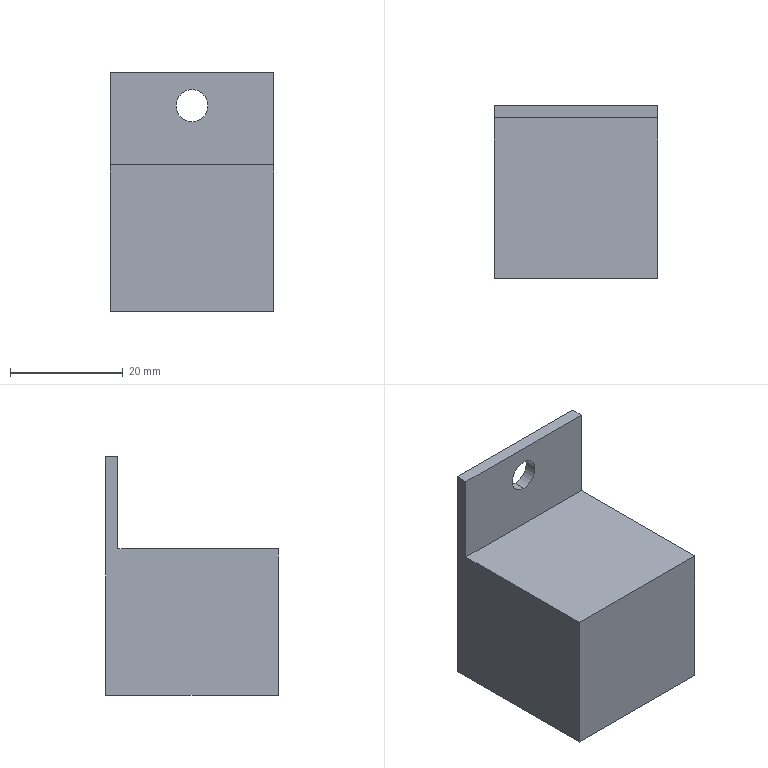Part | SolidWorks | features BaseBody 1 | 1 solid | 10 faces | box 29 x 30.7 x 42.4 mm | volume 24138 mm3 | plane 8 | cylinder 2 | commonest cylinder face diameters 5.7 x2
STEP:
#1=CARTESIAN_POINT('',(62.55,140.,80.3));
#2=VERTEX_POINT('',#1);
#3=CARTESIAN_POINT('',(62.55,140.,86.));
#4=VERTEX_POINT('',#3);
#5=CARTESIAN_POINT('',(62.55,140.,83.15));
#6=DIRECTION('',(0.,1.,0.));
#7=DIRECTION('',(0.,0.,-1.));
#8=AXIS2_PLACEMENT_3D('',#5,#6,#7);
#9=CIRCLE('',#8,2.85);
#10=EDGE_CURVE('',#2,#4,#9,.T.);
#11=ORIENTED_EDGE('',*,*,#10,.T.);
#12=CARTESIAN_POINT('',(62.55,137.8,86.));
#13=VERTEX_POINT('',#12);
#14=CARTESIAN_POINT('',(62.55,151.8,86.));
#15=DIRECTION('',(0.,-1.,0.));
#16=VECTOR('',#15,1000.);
#17=LINE('',#14,#16);
#18=EDGE_CURVE('',#4,#13,#17,.T.);
#19=ORIENTED_EDGE('',*,*,#18,.T.);
#20=CARTESIAN_POINT('',(62.55,137.8,80.3));
#21=VERTEX_POINT('',#20);
#22=CARTESIAN_POINT('',(62.55,137.8,83.15));
#23=DIRECTION('',(0.,1.,0.));
#24=DIRECTION('',(0.,0.,-1.));
#25=AXIS2_PLACEMENT_3D('',#22,#23,#24);
#26=CIRCLE('',#25,2.85);
#27=EDGE_CURVE('',#21,#13,#26,.T.);
#28=ORIENTED_EDGE('',*,*,#27,.F.);
#29=CARTESIAN_POINT('',(62.55,151.8,80.3));
#30=DIRECTION('',(0.,-1.,0.));
#31=VECTOR('',#30,1000.);
#32=LINE('',#29,#31);
#33=EDGE_CURVE('',#2,#21,#32,.T.);
#34=ORIENTED_EDGE('',*,*,#33,.F.);
#35=EDGE_LOOP('',(#11,#19,#28,#34));
#36=FACE_OUTER_BOUND('',#35,.T.);
#37=CARTESIAN_POINT('',(62.55,151.8,83.15));
#38=DIRECTION('',(0.,-1.,0.));
#39=DIRECTION('',(0.,0.,-1.));
#40=AXIS2_PLACEMENT_3D('',#37,#38,#39);
#41=CYLINDRICAL_SURFACE('',#40,2.85);
#42=ADVANCED_FACE('',(#36),#41,.F.);
#43=CARTESIAN_POINT('',(48.05,137.8,72.6));
#44=VERTEX_POINT('',#43);
#45=CARTESIAN_POINT('',(77.05,137.8,72.6));
#46=VERTEX_POINT('',#45);
#47=CARTESIAN_POINT('',(-59.95,137.8,72.6));
#48=DIRECTION('',(1.,0.,0.));
#49=VECTOR('',#48,1000.);
#50=LINE('',#47,#49);
#51=EDGE_CURVE('',#44,#46,#50,.T.);
#52=ORIENTED_EDGE('',*,*,#51,.F.);
#53=CARTESIAN_POINT('',(48.05,109.3,72.6));
#54=VERTEX_POINT('',#53);
#55=CARTESIAN_POINT('',(48.05,140.,72.6));
#56=DIRECTION('',(0.,1.,0.));
#57=VECTOR('',#56,1000.);
#58=LINE('',#55,#57);
#59=EDGE_CURVE('',#54,#44,#58,.T.);
#60=ORIENTED_EDGE('',*,*,#59,.F.);
#61=CARTESIAN_POINT('',(77.05,109.3,72.6));
#62=VERTEX_POINT('',#61);
#63=CARTESIAN_POINT('',(-39.9,109.3,72.6));
#64=DIRECTION('',(-1.,0.,0.));
#65=VECTOR('',#64,1000.);
#66=LINE('',#63,#65);
#67=EDGE_CURVE('',#62,#54,#66,.T.);
#68=ORIENTED_EDGE('',*,*,#67,.F.);
#69=CARTESIAN_POINT('',(77.05,140.,72.6));
#70=DIRECTION('',(0.,-1.,0.));
#71=VECTOR('',#70,1000.);
#72=LINE('',#69,#71);
#73=EDGE_CURVE('',#46,#62,#72,.T.);
#74=ORIENTED_EDGE('',*,*,#73,.F.);
#75=EDGE_LOOP('',(#52,#60,#68,#74));
#76=FACE_OUTER_BOUND('',#75,.T.);
#77=CARTESIAN_POINT('',(48.05,140.,72.6));
#78=DIRECTION('',(0.,0.,1.));
#79=DIRECTION('',(1.,0.,0.));
#80=AXIS2_PLACEMENT_3D('',#77,#78,#79);
#81=PLANE('',#80);
#82=ADVANCED_FACE('',(#76),#81,.T.);
#83=CARTESIAN_POINT('',(77.05,109.3,46.6));
#84=VERTEX_POINT('',#83);
#85=CARTESIAN_POINT('',(77.05,109.3,72.6));
#86=DIRECTION('',(0.,0.,-1.));
#87=VECTOR('',#86,1000.);
#88=LINE('',#85,#87);
#89=EDGE_CURVE('',#62,#84,#88,.T.);
#90=ORIENTED_EDGE('',*,*,#89,.F.);
#91=ORIENTED_EDGE('',*,*,#67,.T.);
#92=CARTESIAN_POINT('',(48.05,109.3,46.6));
#93=VERTEX_POINT('',#92);
#94=CARTESIAN_POINT('',(48.05,109.3,46.6));
#95=DIRECTION('',(0.,0.,1.));
#96=VECTOR('',#95,1000.);
#97=LINE('',#94,#96);
#98=EDGE_CURVE('',#93,#54,#97,.T.);
#99=ORIENTED_EDGE('',*,*,#98,.F.);
#100=CARTESIAN_POINT('',(77.05,109.3,46.6));
#101=DIRECTION('',(-1.,0.,0.));
#102=VECTOR('',#101,1000.);
#103=LINE('',#100,#102);
#104=EDGE_CURVE('',#84,#93,#103,.T.);
#105=ORIENTED_EDGE('',*,*,#104,.F.);
#106=EDGE_LOOP('',(#90,#91,#99,#105));
#107=FACE_OUTER_BOUND('',#106,.T.);
#108=CARTESIAN_POINT('',(-39.9,109.3,-5.4));
#109=DIRECTION('',(0.,-1.,0.));
#110=DIRECTION('',(0.,0.,-1.));
#111=AXIS2_PLACEMENT_3D('',#108,#109,#110);
#112=PLANE('',#111);
#113=ADVANCED_FACE('',(#107),#112,.T.);
#114=ORIENTED_EDGE('',*,*,#27,.T.);
#115=CARTESIAN_POINT('',(62.55,137.8,83.15));
#116=DIRECTION('',(0.,1.,0.));
#117=DIRECTION('',(0.,0.,-1.));
#118=AXIS2_PLACEMENT_3D('',#115,#116,#117);
#119=CIRCLE('',#118,2.85);
#120=EDGE_CURVE('',#13,#21,#119,.T.);
#121=ORIENTED_EDGE('',*,*,#120,.T.);
#122=EDGE_LOOP('',(#114,#121));
#123=FACE_BOUND('',#122,.T.);
#124=CARTESIAN_POINT('',(77.05,137.8,89.));
#125=VERTEX_POINT('',#124);
#126=CARTESIAN_POINT('',(77.05,137.8,72.6));
#127=DIRECTION('',(0.,0.,-1.));
#128=VECTOR('',#127,1000.);
#129=LINE('',#126,#128);
#130=EDGE_CURVE('',#125,#46,#129,.T.);
#131=ORIENTED_EDGE('',*,*,#130,.F.);
#132=CARTESIAN_POINT('',(48.05,137.8,89.));
#133=VERTEX_POINT('',#132);
#134=CARTESIAN_POINT('',(48.05,137.8,89.));
#135=DIRECTION('',(1.,0.,0.));
#136=VECTOR('',#135,1000.);
#137=LINE('',#134,#136);
#138=EDGE_CURVE('',#133,#125,#137,.T.);
#139=ORIENTED_EDGE('',*,*,#138,.F.);
#140=CARTESIAN_POINT('',(48.05,137.8,46.6));
#141=DIRECTION('',(0.,0.,1.));
#142=VECTOR('',#141,1000.);
#143=LINE('',#140,#142);
#144=EDGE_CURVE('',#44,#133,#143,.T.);
#145=ORIENTED_EDGE('',*,*,#144,.F.);
#146=ORIENTED_EDGE('',*,*,#51,.T.);
#147=EDGE_LOOP('',(#131,#139,#145,#146));
#148=FACE_OUTER_BOUND('',#147,.T.);
#149=CARTESIAN_POINT('',(-59.95,137.8,45.6));
#150=DIRECTION('',(0.,-1.,0.));
#151=DIRECTION('',(0.,0.,-1.));
#152=AXIS2_PLACEMENT_3D('',#149,#150,#151);
#153=PLANE('',#152);
#154=ADVANCED_FACE('',(#123,#148),#153,.T.);
#155=CARTESIAN_POINT('',(77.05,140.,89.));
#156=VERTEX_POINT('',#155);
#157=CARTESIAN_POINT('',(77.05,140.,89.));
#158=DIRECTION('',(0.,1.,0.));
#159=VECTOR('',#158,1000.);
#160=LINE('',#157,#159);
#161=EDGE_CURVE('',#125,#156,#160,.T.);
#162=ORIENTED_EDGE('',*,*,#161,.F.);
#163=ORIENTED_EDGE('',*,*,#130,.T.);
#164=ORIENTED_EDGE('',*,*,#73,.T.);
#165=ORIENTED_EDGE('',*,*,#89,.T.);
#166=CARTESIAN_POINT('',(77.05,140.,46.6));
#167=VERTEX_POINT('',#166);
#168=CARTESIAN_POINT('',(77.05,140.,46.6));
#169=DIRECTION('',(0.,-1.,0.));
#170=VECTOR('',#169,1000.);
#171=LINE('',#168,#170);
#172=EDGE_CURVE('',#167,#84,#171,.T.);
#173=ORIENTED_EDGE('',*,*,#172,.F.);
#174=CARTESIAN_POINT('',(77.05,140.,-5.4));
#175=DIRECTION('',(0.,0.,1.));
#176=VECTOR('',#175,1000.);
#177=LINE('',#174,#176);
#178=EDGE_CURVE('',#167,#156,#177,.T.);
#179=ORIENTED_EDGE('',*,*,#178,.T.);
#180=EDGE_LOOP('',(#162,#163,#164,#165,#173,#179));
#181=FACE_OUTER_BOUND('',#180,.T.);
#182=CARTESIAN_POINT('',(77.05,140.,72.6));
#183=DIRECTION('',(1.,0.,0.));
#184=DIRECTION('',(0.,1.,0.));
#185=AXIS2_PLACEMENT_3D('',#182,#183,#184);
#186=PLANE('',#185);
#187=ADVANCED_FACE('',(#181),#186,.T.);
#188=ORIENTED_EDGE('',*,*,#161,.T.);
#189=CARTESIAN_POINT('',(48.05,140.,89.));
#190=VERTEX_POINT('',#189);
#191=CARTESIAN_POINT('',(-39.9,140.,89.));
#192=DIRECTION('',(-1.,0.,0.));
#193=VECTOR('',#192,1000.);
#194=LINE('',#191,#193);
#195=EDGE_CURVE('',#156,#190,#194,.T.);
#196=ORIENTED_EDGE('',*,*,#195,.T.);
#197=CARTESIAN_POINT('',(48.05,140.,89.));
#198=DIRECTION('',(0.,1.,0.));
#199=VECTOR('',#198,1000.);
#200=LINE('',#197,#199);
#201=EDGE_CURVE('',#133,#190,#200,.T.);
#202=ORIENTED_EDGE('',*,*,#201,.F.);
#203=ORIENTED_EDGE('',*,*,#138,.T.);
#204=EDGE_LOOP('',(#188,#196,#202,#203));
#205=FACE_OUTER_BOUND('',#204,.T.);
#206=CARTESIAN_POINT('',(48.05,140.,89.));
#207=DIRECTION('',(0.,0.,1.));
#208=DIRECTION('',(1.,0.,0.));
#209=AXIS2_PLACEMENT_3D('',#206,#207,#208);
#210=PLANE('',#209);
#211=ADVANCED_FACE('',(#205),#210,.T.);
#212=CARTESIAN_POINT('',(48.05,140.,46.6));
#213=VERTEX_POINT('',#212);
#214=CARTESIAN_POINT('',(48.05,140.,46.6));
#215=DIRECTION('',(0.,1.,0.));
#216=VECTOR('',#215,1000.);
#217=LINE('',#214,#216);
#218=EDGE_CURVE('',#93,#213,#217,.T.);
#219=ORIENTED_EDGE('',*,*,#218,.F.);
#220=ORIENTED_EDGE('',*,*,#98,.T.);
#221=ORIENTED_EDGE('',*,*,#59,.T.);
#222=ORIENTED_EDGE('',*,*,#144,.T.);
#223=ORIENTED_EDGE('',*,*,#201,.T.);
#224=CARTESIAN_POINT('',(48.05,140.,-5.4));
#225=DIRECTION('',(0.,0.,-1.));
#226=VECTOR('',#225,1000.);
#227=LINE('',#224,#226);
#228=EDGE_CURVE('',#190,#213,#227,.T.);
#229=ORIENTED_EDGE('',*,*,#228,.T.);
#230=EDGE_LOOP('',(#219,#220,#221,#222,#223,#229));
#231=FACE_OUTER_BOUND('',#230,.T.);
#232=CARTESIAN_POINT('',(48.05,140.,46.6));
#233=DIRECTION('',(-1.,0.,0.));
#234=DIRECTION('',(0.,0.,1.));
#235=AXIS2_PLACEMENT_3D('',#232,#233,#234);
#236=PLANE('',#235);
#237=ADVANCED_FACE('',(#231),#236,.T.);
#238=ORIENTED_EDGE('',*,*,#218,.T.);
#239=CARTESIAN_POINT('',(-39.9,140.,46.6));
#240=DIRECTION('',(1.,0.,0.));
#241=VECTOR('',#240,1000.);
#242=LINE('',#239,#241);
#243=EDGE_CURVE('',#213,#167,#242,.T.);
#244=ORIENTED_EDGE('',*,*,#243,.T.);
#245=ORIENTED_EDGE('',*,*,#172,.T.);
#246=ORIENTED_EDGE('',*,*,#104,.T.);
#247=EDGE_LOOP('',(#238,#244,#245,#246));
#248=FACE_OUTER_BOUND('',#247,.T.);
#249=CARTESIAN_POINT('',(77.05,140.,46.6));
#250=DIRECTION('',(0.,0.,-1.));
#251=DIRECTION('',(0.,-1.,0.));
#252=AXIS2_PLACEMENT_3D('',#249,#250,#251);
#253=PLANE('',#252);
#254=ADVANCED_FACE('',(#248),#253,.T.);
#255=ORIENTED_EDGE('',*,*,#10,.F.);
#256=CARTESIAN_POINT('',(62.55,140.,83.15));
#257=DIRECTION('',(0.,1.,0.));
#258=DIRECTION('',(0.,0.,-1.));
#259=AXIS2_PLACEMENT_3D('',#256,#257,#258);
#260=CIRCLE('',#259,2.85);
#261=EDGE_CURVE('',#4,#2,#260,.T.);
#262=ORIENTED_EDGE('',*,*,#261,.F.);
#263=EDGE_LOOP('',(#255,#262));
#264=FACE_BOUND('',#263,.T.);
#265=ORIENTED_EDGE('',*,*,#228,.F.);
#266=ORIENTED_EDGE('',*,*,#195,.F.);
#267=ORIENTED_EDGE('',*,*,#178,.F.);
#268=ORIENTED_EDGE('',*,*,#243,.F.);
#269=EDGE_LOOP('',(#265,#266,#267,#268));
#270=FACE_OUTER_BOUND('',#269,.T.);
#271=CARTESIAN_POINT('',(-39.9,140.,-5.4));
#272=DIRECTION('',(0.,-1.,0.));
#273=DIRECTION('',(0.,0.,-1.));
#274=AXIS2_PLACEMENT_3D('',#271,#272,#273);
#275=PLANE('',#274);
#276=ADVANCED_FACE('',(#264,#270),#275,.F.);
#277=ORIENTED_EDGE('',*,*,#18,.F.);
#278=ORIENTED_EDGE('',*,*,#261,.T.);
#279=ORIENTED_EDGE('',*,*,#33,.T.);
#280=ORIENTED_EDGE('',*,*,#120,.F.);
#281=EDGE_LOOP('',(#277,#278,#279,#280));
#282=FACE_OUTER_BOUND('',#281,.T.);
#283=CARTESIAN_POINT('',(62.55,151.8,83.15));
#284=DIRECTION('',(0.,-1.,0.));
#285=DIRECTION('',(0.,0.,-1.));
#286=AXIS2_PLACEMENT_3D('',#283,#284,#285);
#287=CYLINDRICAL_SURFACE('',#286,2.85);
#288=ADVANCED_FACE('',(#282),#287,.F.);
#289=CLOSED_SHELL('',(#42,#82,#113,#154,#187,#211,#237,#254,#276,#288));
#290=MANIFOLD_SOLID_BREP('',#289);
#291=CARTESIAN_POINT('',(0.,0.,0.));
#292=DIRECTION('',(0.,0.,1.));
#293=DIRECTION('',(1.,0.,0.));
#294=AXIS2_PLACEMENT_3D('',#291,#292,#293);
#295=(LENGTH_UNIT()NAMED_UNIT(*)SI_UNIT(.MILLI.,.METRE.));
#296=UNCERTAINTY_MEASURE_WITH_UNIT(LENGTH_MEASURE(0.00001),#295,'','');
#297=(NAMED_UNIT(*)PLANE_ANGLE_UNIT()SI_UNIT($,.RADIAN.));
#298=(NAMED_UNIT(*)SI_UNIT($,.STERADIAN.)SOLID_ANGLE_UNIT());
#299=(GEOMETRIC_REPRESENTATION_CONTEXT(3)GLOBAL_UNCERTAINTY_ASSIGNED_CONTEXT((#296))GLOBAL_UNIT_ASSIGNED_CONTEXT((#295,#297,#298))REPRESENTATION_CONTEXT('',''));
#300=ADVANCED_BREP_SHAPE_REPRESENTATION('',(#290,#294),#299);